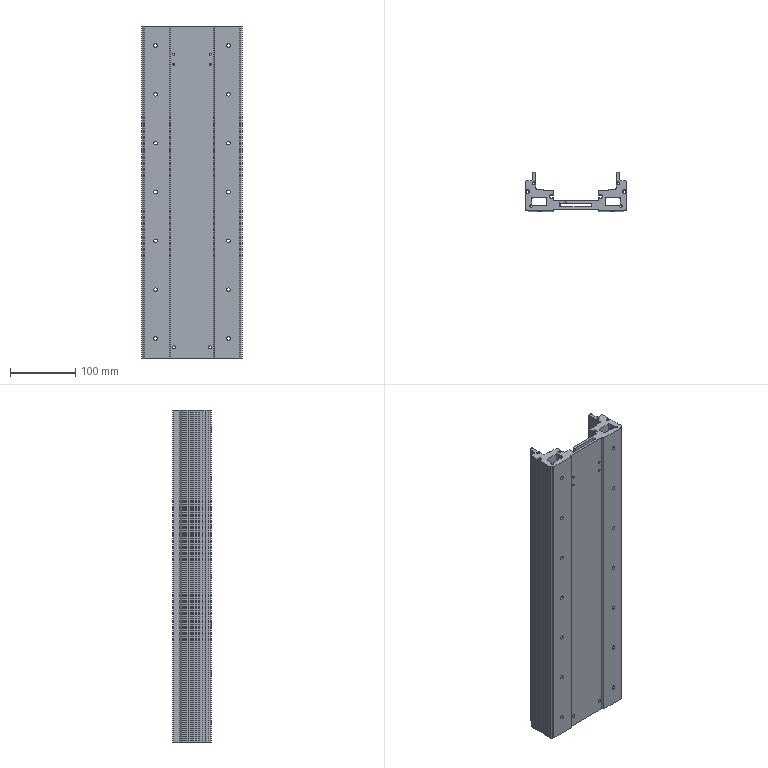Part | STEP file | 1 solid | 307 faces | box 155 x 59.25 x 510 mm | volume 1638081 mm3 | plane 166 | cylinder 119 | cone 22 | commonest cylinder face diameters 3.3 x22 5 x18 5.5 x14 9 x14 2 x12 0.5 x8